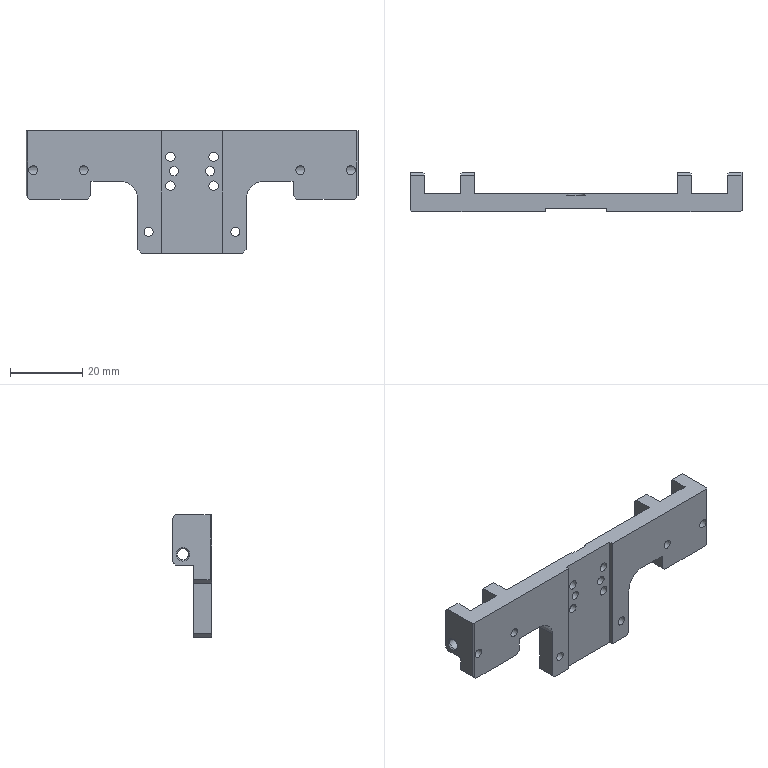CAM job | NX | 3+2 milling, drilling | part box 92 x 11 x 34 mm | stock box 97 x 15 x 35 mm
Tools:
number,name,description,diameter,corner_radius,flute_length,length,flutes
3,D3,平底铣刀-粗,3.0,0.0,20.0,75.0,2
8,D8,平底铣刀-粗,8.0,0.0,30.0,75.0,2
9,D10,平底铣刀-粗,10.0,0.0,35.0,75.0,2
11,D3-J,平底铣刀-精,3.0,0.0,50.0,75.0,2
7,D6-J,平底铣刀-精,6.0,0.0,25.0,75.0,2
1,D80R0.8飞刀,圆鼻刀-粗,80.0,0.8,50.0,75.0,2
1,D80R0.8飞刀-J,圆鼻刀-精,80.0,0.8,50.0,75.0,2
2,D6倒角刀,倒角刀,6.0,0.0,3.0,25.0,2
20,M3X0.5,丝锥,2.5,0.0,35.0,50.0,2
12,ZT2.6,钻头,2.6,0.0,35.0,50.0,2
Operations:
program,operation,operation_type,tool,method,geometry_group,spindle_rpm,surface_speed,feed_per_tooth,feed_cut,feed_plunge,cut_length_mm,path_length_mm,cut_time_min,machine_time_min
B,BOTWALLFLYCUTROUGH_COPY,VolumeBased25DMillingOperation,D80R0.8飞刀,ZLEVELROUGH-DEPTHK-STEPG,W-B,2800.0,703.696,0.5357,3000.0,100.0,1401.358,2714.438,0.4671,0.5984
B,BOTWALLFLYCUTFINISH_COPY,VolumeBased25DMillingOperation,D80R0.8飞刀-J,SIDEFINISH-DEPTHK-STEPG,W-B,4000.0,1005.28,0.125,1000.0,100.0,199.998,235.998,0.2,0.2036
B,BOTWALLZROUGH-MID_COPY,VolumeBased25DMillingOperation,D8,ZLEVELROUGH-DEPTHK-STEPG,W-B,8000.0,251.32,0.25,4000.0,100.0,6040.555,6233.914,1.51,1.53
B,CSINKMILL_1,CylinderMilling,D3,METHOD,W-B,8000.0,75.398,0.0688,1100.0,100.0,122.751,305.551,0.1116,0.1299
B,CSINKMILL_2,CylinderMilling,D3,METHOD,W-B,8000.0,100.531,0.075,1200.0,100.0,211.651,455.651,0.1764,0.2008
B,BOTWALLZROUGH-MID_COPY_1,VolumeBased25DMillingOperation,D3,ZLEVELROUGH-DEPTHK-STEPG,W-B,8000.0,75.398,0.0625,1000.0,100.0,50.913,89.324,0.0509,0.0548
B,DRILLCHAMFER_3,Operation,D6倒角刀,METHOD,W-B,8000.0,150.796,0.0625,1000.0,0.0,19.0,146.24,0.019,0.0317
B,FACEDEBURR6X45L_COPY,SurfaceContour,D6倒角刀,CLIMBCHAMFER-DEPTH0-STEPG,W-B,6500.0,122.519,0.1154,1500.0,100.0,391.92,1038.289,0.2613,0.3259
B,BOTWALLCHAMFER_COPY,VolumeBased25DMillingOperation,D6倒角刀,CLIMBCHAMFER-DEPTH0-STEPG,W-B,6500.0,122.519,0.1154,1500.0,100.0,174.401,496.644,0.1163,0.1485
B,BOTWALLFINISHFLOOR-MID_COPY,VolumeBased25DMillingOperation,D6-J,FINISH-STEPDEPTH-OFF,W-B,8000.0,150.792,0.0625,1000.0,100.0,737.56,898.027,0.7376,0.7536
B,BOTWALLFINISHWALL-MID-SELFLOOR_COPY,VolumeBased25DMillingOperation,D6-J,SIDEFINISH-DEPTHK-STEPG,W-B,8000.0,150.792,0.0625,1000.0,100.0,183.078,267.279,0.1831,0.1915
B,HOLEMILL_1,CylinderMilling,D3-J,METHOD,W-B,8000.0,75.398,0.0187,300.0,100.0,12.005,202.005,0.04,0.059
B,HOLEMILL_2,CylinderMilling,D3-J,METHOD,W-B,8000.0,100.531,0.0375,600.0,100.0,25.506,279.906,0.0425,0.068
B,BOTWALLFINISHWALL-MID-SELFLOOR_COPY_1,VolumeBased25DMillingOperation,D3-J,SIDEFINISH-DEPTHK-STEPG,W-B,8000.0,100.528,0.05,800.0,100.0,20.855,58.855,0.0261,0.0299
A,TOPFACE,FaceMilling,D80R0.8飞刀,SIDEFINISH-DEPTHK-STEPG,W-A,4000.0,1005.31,0.125,1000.0,100.0,186.0,222.0,0.186,0.1896
A,ADAPTIVEROUGHD10_COPY,CavityMilling,D10,ADAPTIVE-DEPTHK-STEPK,W-A,8000.0,251.32,0.25,4000.0,100.0,2694.781,2852.418,0.6737,0.6895
A,BOTWALLROUGH_1,VolumeBased25DMillingOperation,D10,METHOD,W-A,6000.0,113.0,0.2083,3500.0,100.0,188.2,236.918,0.0538,0.0586
A,SPOTDRILL-DEPTH0.8,Operation,D6倒角刀,NONE,W-A,8000.0,150.796,0.0312,500.0,90.0,21.6,229.165,0.0432,0.064
A,THRUHOLE-2-3,Operation,ZT2.6,NONE,W-A,3000.0,24.504,0.0133,80.0,90.0,21.924,117.015,0.2741,0.2836
A,THRUHOLE-M3TAPDRILL,Operation,ZT2.6,NONE,W-A,3000.0,23.562,0.05,300.0,90.0,46.0,181.467,0.1533,0.1669
A,BLINDCONEHOLE-M3TAPDRILL,Operation,ZT2.6,NONE,W-A,3000.0,23.562,0.0167,100.0,90.0,39.2,209.48,0.392,0.409
A,BOTFINISH_1,VolumeBased25DMillingOperation,D6-J,METHOD,W-A,6000.0,113.0,0.2083,1200.0,100.0,169.5,210.5,0.1413,0.1454
A,PROFILESIDE,ZLevelMilling,D3-J,METHOD,W-A,9000.0,84.823,0.1389,2500.0,80.0,856.736,1002.85,0.3429,0.3575
A,SELBODYONLY,SurfaceContour,D6倒角刀,METHOD,W-A,8000.0,150.796,0.1875,3000.0,100.0,279.265,618.22,0.0931,0.127
A,DRILLCHAMFER_1,Operation,D6倒角刀,METHOD,W-A,8000.0,150.796,0.0312,500.0,0.0,38.0,262.809,0.076,0.0985
A,DRILLCHAMFER_2,Operation,D6倒角刀,METHOD,W-A,8000.0,150.796,0.0312,500.0,0.0,18.4,117.257,0.0368,0.0467
A,THRUHOLE-TAPM3,Operation,M3X0.5,METHOD,W-A,800.0,6.283,0.0003,0.5,90.0,36.0,161.413,72.0,72.013
A,BLINDCONEHOLE-TAPM3,Operation,M3X0.5,METHOD,W-A,1000.0,7.854,0.0003,0.5,90.0,36.334,203.748,72.668,72.685
A,BOTSIDEFINISH_3,VolumeBased25DMillingOperation,D6-J,METHOD,W-A,6000.0,113.0,0.2083,1200.0,100.0,87.483,178.323,0.0729,0.082
A,PROFILESEMIFINISH_2,VolumeBased25DMillingOperation,D6-J,METHOD,W-A,8000.0,251.327,0.0625,1000.0,100.0,285.384,346.384,0.2854,0.2915